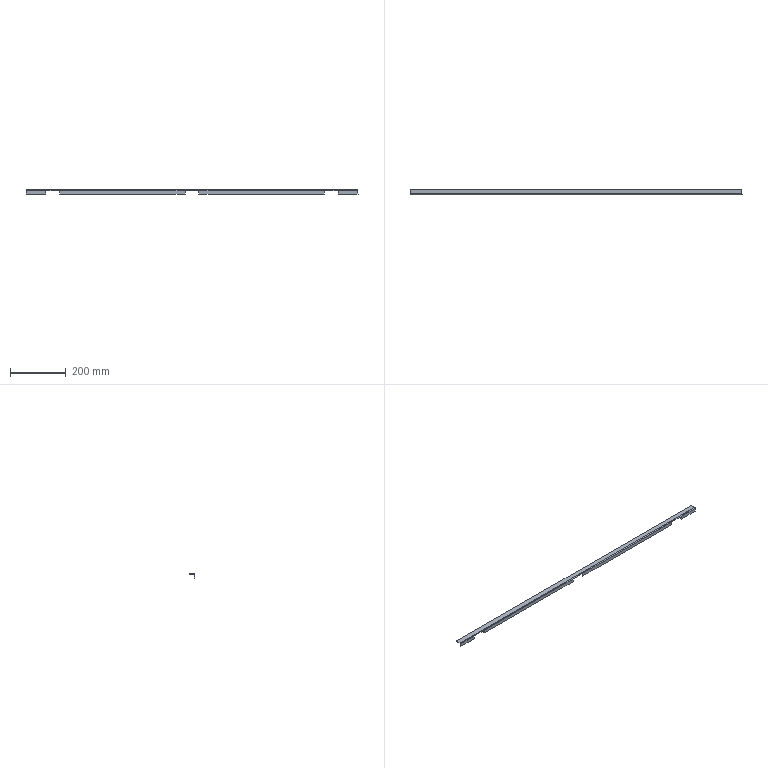Part | SolidWorks | features LPattern 2, Cut 1, EdgeFlange 1, FlatPattern 1, ICE 1, SMBaseFlange 1, SheetMetal 1 | 1 solid | 32 faces | box 1191 x 20 x 15 mm | volume 90032 mm3 | plane 30 | cylinder 2 | commonest cylinder face diameters 1 x1 6 x1
STEP:
#1=CARTESIAN_POINT('',(475.,-10.,-3.));
#2=VERTEX_POINT('',#1);
#3=CARTESIAN_POINT('',(25.,-10.,-3.));
#4=VERTEX_POINT('',#3);
#5=CARTESIAN_POINT('',(-595.5,-10.,-3.));
#6=DIRECTION('',(-1.,0.,0.));
#7=VECTOR('',#6,1000.);
#8=LINE('',#5,#7);
#9=EDGE_CURVE('',#2,#4,#8,.T.);
#10=ORIENTED_EDGE('',*,*,#9,.T.);
#11=CARTESIAN_POINT('',(25.,-10.,-15.));
#12=VERTEX_POINT('',#11);
#13=CARTESIAN_POINT('',(25.,-10.,-2.5));
#14=DIRECTION('',(0.,0.,-1.));
#15=VECTOR('',#14,1000.);
#16=LINE('',#13,#15);
#17=EDGE_CURVE('',#4,#12,#16,.T.);
#18=ORIENTED_EDGE('',*,*,#17,.T.);
#19=CARTESIAN_POINT('',(475.,-10.,-15.));
#20=VERTEX_POINT('',#19);
#21=CARTESIAN_POINT('',(-595.5,-10.,-15.));
#22=DIRECTION('',(-1.,0.,0.));
#23=VECTOR('',#22,1000.);
#24=LINE('',#21,#23);
#25=EDGE_CURVE('',#20,#12,#24,.T.);
#26=ORIENTED_EDGE('',*,*,#25,.F.);
#27=CARTESIAN_POINT('',(475.,-10.,-2.5));
#28=DIRECTION('',(0.,0.,1.));
#29=VECTOR('',#28,1000.);
#30=LINE('',#27,#29);
#31=EDGE_CURVE('',#20,#2,#30,.T.);
#32=ORIENTED_EDGE('',*,*,#31,.T.);
#33=EDGE_LOOP('',(#10,#18,#26,#32));
#34=FACE_OUTER_BOUND('',#33,.T.);
#35=CARTESIAN_POINT('',(-595.5,-10.,-2.5));
#36=DIRECTION('',(0.,-1.,0.));
#37=DIRECTION('',(0.,0.,-1.));
#38=AXIS2_PLACEMENT_3D('',#35,#36,#37);
#39=PLANE('',#38);
#40=ADVANCED_FACE('',(#34),#39,.T.);
#41=CARTESIAN_POINT('',(-25.,-10.,-15.));
#42=VERTEX_POINT('',#41);
#43=CARTESIAN_POINT('',(-475.,-10.,-15.));
#44=VERTEX_POINT('',#43);
#45=CARTESIAN_POINT('',(-595.5,-10.,-15.));
#46=DIRECTION('',(-1.,0.,0.));
#47=VECTOR('',#46,1000.);
#48=LINE('',#45,#47);
#49=EDGE_CURVE('',#42,#44,#48,.T.);
#50=ORIENTED_EDGE('',*,*,#49,.F.);
#51=CARTESIAN_POINT('',(-25.,-10.,-3.));
#52=VERTEX_POINT('',#51);
#53=CARTESIAN_POINT('',(-25.,-10.,-2.5));
#54=DIRECTION('',(0.,0.,1.));
#55=VECTOR('',#54,1000.);
#56=LINE('',#53,#55);
#57=EDGE_CURVE('',#42,#52,#56,.T.);
#58=ORIENTED_EDGE('',*,*,#57,.T.);
#59=CARTESIAN_POINT('',(-475.,-10.,-3.));
#60=VERTEX_POINT('',#59);
#61=CARTESIAN_POINT('',(-595.5,-10.,-3.));
#62=DIRECTION('',(-1.,0.,0.));
#63=VECTOR('',#62,1000.);
#64=LINE('',#61,#63);
#65=EDGE_CURVE('',#52,#60,#64,.T.);
#66=ORIENTED_EDGE('',*,*,#65,.T.);
#67=CARTESIAN_POINT('',(-475.,-10.,-2.5));
#68=DIRECTION('',(0.,0.,-1.));
#69=VECTOR('',#68,1000.);
#70=LINE('',#67,#69);
#71=EDGE_CURVE('',#60,#44,#70,.T.);
#72=ORIENTED_EDGE('',*,*,#71,.T.);
#73=EDGE_LOOP('',(#50,#58,#66,#72));
#74=FACE_OUTER_BOUND('',#73,.T.);
#75=CARTESIAN_POINT('',(-595.5,-10.,-2.5));
#76=DIRECTION('',(0.,-1.,0.));
#77=DIRECTION('',(0.,0.,-1.));
#78=AXIS2_PLACEMENT_3D('',#75,#76,#77);
#79=PLANE('',#78);
#80=ADVANCED_FACE('',(#74),#79,.T.);
#81=CARTESIAN_POINT('',(25.,-7.5,-3.));
#82=VERTEX_POINT('',#81);
#83=CARTESIAN_POINT('',(25.,-7.5,-15.));
#84=VERTEX_POINT('',#83);
#85=CARTESIAN_POINT('',(25.,-7.5,-3.));
#86=DIRECTION('',(0.,0.,-1.));
#87=VECTOR('',#86,1000.);
#88=LINE('',#85,#87);
#89=EDGE_CURVE('',#82,#84,#88,.T.);
#90=ORIENTED_EDGE('',*,*,#89,.F.);
#91=CARTESIAN_POINT('',(475.,-7.5,-3.));
#92=VERTEX_POINT('',#91);
#93=CARTESIAN_POINT('',(595.5,-7.5,-3.));
#94=DIRECTION('',(-1.,0.,0.));
#95=VECTOR('',#94,1000.);
#96=LINE('',#93,#95);
#97=EDGE_CURVE('',#92,#82,#96,.T.);
#98=ORIENTED_EDGE('',*,*,#97,.F.);
#99=CARTESIAN_POINT('',(475.,-7.5,-15.));
#100=VERTEX_POINT('',#99);
#101=CARTESIAN_POINT('',(475.,-7.5,-3.));
#102=DIRECTION('',(0.,0.,1.));
#103=VECTOR('',#102,1000.);
#104=LINE('',#101,#103);
#105=EDGE_CURVE('',#100,#92,#104,.T.);
#106=ORIENTED_EDGE('',*,*,#105,.F.);
#107=CARTESIAN_POINT('',(-595.5,-7.5,-15.));
#108=DIRECTION('',(-1.,0.,0.));
#109=VECTOR('',#108,1000.);
#110=LINE('',#107,#109);
#111=EDGE_CURVE('',#100,#84,#110,.T.);
#112=ORIENTED_EDGE('',*,*,#111,.T.);
#113=EDGE_LOOP('',(#90,#98,#106,#112));
#114=FACE_OUTER_BOUND('',#113,.T.);
#115=CARTESIAN_POINT('',(-595.5,-7.5,-2.5));
#116=DIRECTION('',(0.,-1.,0.));
#117=DIRECTION('',(0.,0.,-1.));
#118=AXIS2_PLACEMENT_3D('',#115,#116,#117);
#119=PLANE('',#118);
#120=ADVANCED_FACE('',(#114),#119,.F.);
#121=CARTESIAN_POINT('',(-25.,-7.5,-15.));
#122=VERTEX_POINT('',#121);
#123=CARTESIAN_POINT('',(-25.,-7.5,-3.));
#124=VERTEX_POINT('',#123);
#125=CARTESIAN_POINT('',(-25.,-7.5,-3.));
#126=DIRECTION('',(0.,0.,1.));
#127=VECTOR('',#126,1000.);
#128=LINE('',#125,#127);
#129=EDGE_CURVE('',#122,#124,#128,.T.);
#130=ORIENTED_EDGE('',*,*,#129,.F.);
#131=CARTESIAN_POINT('',(-475.,-7.5,-15.));
#132=VERTEX_POINT('',#131);
#133=CARTESIAN_POINT('',(-595.5,-7.5,-15.));
#134=DIRECTION('',(-1.,0.,0.));
#135=VECTOR('',#134,1000.);
#136=LINE('',#133,#135);
#137=EDGE_CURVE('',#122,#132,#136,.T.);
#138=ORIENTED_EDGE('',*,*,#137,.T.);
#139=CARTESIAN_POINT('',(-475.,-7.5,-3.));
#140=VERTEX_POINT('',#139);
#141=CARTESIAN_POINT('',(-475.,-7.5,-3.));
#142=DIRECTION('',(0.,0.,-1.));
#143=VECTOR('',#142,1000.);
#144=LINE('',#141,#143);
#145=EDGE_CURVE('',#140,#132,#144,.T.);
#146=ORIENTED_EDGE('',*,*,#145,.F.);
#147=CARTESIAN_POINT('',(595.5,-7.5,-3.));
#148=DIRECTION('',(-1.,0.,0.));
#149=VECTOR('',#148,1000.);
#150=LINE('',#147,#149);
#151=EDGE_CURVE('',#124,#140,#150,.T.);
#152=ORIENTED_EDGE('',*,*,#151,.F.);
#153=EDGE_LOOP('',(#130,#138,#146,#152));
#154=FACE_OUTER_BOUND('',#153,.T.);
#155=CARTESIAN_POINT('',(-595.5,-7.5,-2.5));
#156=DIRECTION('',(0.,-1.,0.));
#157=DIRECTION('',(0.,0.,-1.));
#158=AXIS2_PLACEMENT_3D('',#155,#156,#157);
#159=PLANE('',#158);
#160=ADVANCED_FACE('',(#154),#159,.F.);
#161=ORIENTED_EDGE('',*,*,#25,.T.);
#162=CARTESIAN_POINT('',(25.,-7.5,-15.));
#163=DIRECTION('',(0.,-1.,0.));
#164=VECTOR('',#163,1000.);
#165=LINE('',#162,#164);
#166=EDGE_CURVE('',#84,#12,#165,.T.);
#167=ORIENTED_EDGE('',*,*,#166,.F.);
#168=ORIENTED_EDGE('',*,*,#111,.F.);
#169=CARTESIAN_POINT('',(475.,-7.5,-15.));
#170=DIRECTION('',(0.,-1.,0.));
#171=VECTOR('',#170,1000.);
#172=LINE('',#169,#171);
#173=EDGE_CURVE('',#100,#20,#172,.T.);
#174=ORIENTED_EDGE('',*,*,#173,.T.);
#175=EDGE_LOOP('',(#161,#167,#168,#174));
#176=FACE_OUTER_BOUND('',#175,.T.);
#177=CARTESIAN_POINT('',(-595.5,-10.,-15.));
#178=DIRECTION('',(0.,0.,-1.));
#179=DIRECTION('',(0.,1.,0.));
#180=AXIS2_PLACEMENT_3D('',#177,#178,#179);
#181=PLANE('',#180);
#182=ADVANCED_FACE('',(#176),#181,.T.);
#183=ORIENTED_EDGE('',*,*,#137,.F.);
#184=CARTESIAN_POINT('',(-25.,-7.5,-15.));
#185=DIRECTION('',(0.,-1.,0.));
#186=VECTOR('',#185,1000.);
#187=LINE('',#184,#186);
#188=EDGE_CURVE('',#122,#42,#187,.T.);
#189=ORIENTED_EDGE('',*,*,#188,.T.);
#190=ORIENTED_EDGE('',*,*,#49,.T.);
#191=CARTESIAN_POINT('',(-475.,-7.5,-15.));
#192=DIRECTION('',(0.,-1.,0.));
#193=VECTOR('',#192,1000.);
#194=LINE('',#191,#193);
#195=EDGE_CURVE('',#132,#44,#194,.T.);
#196=ORIENTED_EDGE('',*,*,#195,.F.);
#197=EDGE_LOOP('',(#183,#189,#190,#196));
#198=FACE_OUTER_BOUND('',#197,.T.);
#199=CARTESIAN_POINT('',(-595.5,-10.,-15.));
#200=DIRECTION('',(0.,0.,-1.));
#201=DIRECTION('',(0.,1.,0.));
#202=AXIS2_PLACEMENT_3D('',#199,#200,#201);
#203=PLANE('',#202);
#204=ADVANCED_FACE('',(#198),#203,.T.);
#205=CARTESIAN_POINT('',(595.5,-10.,-3.));
#206=VERTEX_POINT('',#205);
#207=CARTESIAN_POINT('',(525.,-10.,-3.));
#208=VERTEX_POINT('',#207);
#209=CARTESIAN_POINT('',(-595.5,-10.,-3.));
#210=DIRECTION('',(-1.,0.,0.));
#211=VECTOR('',#210,1000.);
#212=LINE('',#209,#211);
#213=EDGE_CURVE('',#206,#208,#212,.T.);
#214=ORIENTED_EDGE('',*,*,#213,.T.);
#215=CARTESIAN_POINT('',(525.,-10.,-15.));
#216=VERTEX_POINT('',#215);
#217=CARTESIAN_POINT('',(525.,-10.,-2.5));
#218=DIRECTION('',(0.,0.,-1.));
#219=VECTOR('',#218,1000.);
#220=LINE('',#217,#219);
#221=EDGE_CURVE('',#208,#216,#220,.T.);
#222=ORIENTED_EDGE('',*,*,#221,.T.);
#223=CARTESIAN_POINT('',(595.5,-10.,-15.));
#224=VERTEX_POINT('',#223);
#225=CARTESIAN_POINT('',(-595.5,-10.,-15.));
#226=DIRECTION('',(-1.,0.,0.));
#227=VECTOR('',#226,1000.);
#228=LINE('',#225,#227);
#229=EDGE_CURVE('',#224,#216,#228,.T.);
#230=ORIENTED_EDGE('',*,*,#229,.F.);
#231=CARTESIAN_POINT('',(595.5,-10.,-15.));
#232=DIRECTION('',(0.,0.,-1.));
#233=VECTOR('',#232,1000.);
#234=LINE('',#231,#233);
#235=EDGE_CURVE('',#206,#224,#234,.T.);
#236=ORIENTED_EDGE('',*,*,#235,.F.);
#237=EDGE_LOOP('',(#214,#222,#230,#236));
#238=FACE_OUTER_BOUND('',#237,.T.);
#239=CARTESIAN_POINT('',(-595.5,-10.,-2.5));
#240=DIRECTION('',(0.,-1.,0.));
#241=DIRECTION('',(0.,0.,-1.));
#242=AXIS2_PLACEMENT_3D('',#239,#240,#241);
#243=PLANE('',#242);
#244=ADVANCED_FACE('',(#238),#243,.T.);
#245=CARTESIAN_POINT('',(525.,-7.5,-3.));
#246=VERTEX_POINT('',#245);
#247=CARTESIAN_POINT('',(525.,-7.5,-15.));
#248=VERTEX_POINT('',#247);
#249=CARTESIAN_POINT('',(525.,-7.5,-3.));
#250=DIRECTION('',(0.,0.,-1.));
#251=VECTOR('',#250,1000.);
#252=LINE('',#249,#251);
#253=EDGE_CURVE('',#246,#248,#252,.T.);
#254=ORIENTED_EDGE('',*,*,#253,.F.);
#255=CARTESIAN_POINT('',(595.5,-7.5,-3.));
#256=VERTEX_POINT('',#255);
#257=CARTESIAN_POINT('',(595.5,-7.5,-3.));
#258=DIRECTION('',(-1.,0.,0.));
#259=VECTOR('',#258,1000.);
#260=LINE('',#257,#259);
#261=EDGE_CURVE('',#256,#246,#260,.T.);
#262=ORIENTED_EDGE('',*,*,#261,.F.);
#263=CARTESIAN_POINT('',(595.5,-7.5,-15.));
#264=VERTEX_POINT('',#263);
#265=CARTESIAN_POINT('',(595.5,-7.5,-2.5));
#266=DIRECTION('',(0.,0.,-1.));
#267=VECTOR('',#266,1000.);
#268=LINE('',#265,#267);
#269=EDGE_CURVE('',#256,#264,#268,.T.);
#270=ORIENTED_EDGE('',*,*,#269,.T.);
#271=CARTESIAN_POINT('',(-595.5,-7.5,-15.));
#272=DIRECTION('',(-1.,0.,0.));
#273=VECTOR('',#272,1000.);
#274=LINE('',#271,#273);
#275=EDGE_CURVE('',#264,#248,#274,.T.);
#276=ORIENTED_EDGE('',*,*,#275,.T.);
#277=EDGE_LOOP('',(#254,#262,#270,#276));
#278=FACE_OUTER_BOUND('',#277,.T.);
#279=CARTESIAN_POINT('',(-595.5,-7.5,-2.5));
#280=DIRECTION('',(0.,-1.,0.));
#281=DIRECTION('',(0.,0.,-1.));
#282=AXIS2_PLACEMENT_3D('',#279,#280,#281);
#283=PLANE('',#282);
#284=ADVANCED_FACE('',(#278),#283,.F.);
#285=ORIENTED_EDGE('',*,*,#229,.T.);
#286=CARTESIAN_POINT('',(525.,-7.5,-15.));
#287=DIRECTION('',(0.,-1.,0.));
#288=VECTOR('',#287,1000.);
#289=LINE('',#286,#288);
#290=EDGE_CURVE('',#248,#216,#289,.T.);
#291=ORIENTED_EDGE('',*,*,#290,.F.);
#292=ORIENTED_EDGE('',*,*,#275,.F.);
#293=CARTESIAN_POINT('',(595.5,-10.,-15.));
#294=DIRECTION('',(0.,1.,0.));
#295=VECTOR('',#294,1000.);
#296=LINE('',#293,#295);
#297=EDGE_CURVE('',#224,#264,#296,.T.);
#298=ORIENTED_EDGE('',*,*,#297,.F.);
#299=EDGE_LOOP('',(#285,#291,#292,#298));
#300=FACE_OUTER_BOUND('',#299,.T.);
#301=CARTESIAN_POINT('',(-595.5,-10.,-15.));
#302=DIRECTION('',(0.,0.,-1.));
#303=DIRECTION('',(0.,1.,0.));
#304=AXIS2_PLACEMENT_3D('',#301,#302,#303);
#305=PLANE('',#304);
#306=ADVANCED_FACE('',(#300),#305,.T.);
#307=CARTESIAN_POINT('',(-525.,-10.,-15.));
#308=VERTEX_POINT('',#307);
#309=CARTESIAN_POINT('',(-595.5,-10.,-15.));
#310=VERTEX_POINT('',#309);
#311=CARTESIAN_POINT('',(-595.5,-10.,-15.));
#312=DIRECTION('',(-1.,0.,0.));
#313=VECTOR('',#312,1000.);
#314=LINE('',#311,#313);
#315=EDGE_CURVE('',#308,#310,#314,.T.);
#316=ORIENTED_EDGE('',*,*,#315,.F.);
#317=CARTESIAN_POINT('',(-525.,-10.,-3.));
#318=VERTEX_POINT('',#317);
#319=CARTESIAN_POINT('',(-525.,-10.,-2.5));
#320=DIRECTION('',(0.,0.,1.));
#321=VECTOR('',#320,1000.);
#322=LINE('',#319,#321);
#323=EDGE_CURVE('',#308,#318,#322,.T.);
#324=ORIENTED_EDGE('',*,*,#323,.T.);
#325=CARTESIAN_POINT('',(-595.5,-10.,-3.));
#326=VERTEX_POINT('',#325);
#327=CARTESIAN_POINT('',(-595.5,-10.,-3.));
#328=DIRECTION('',(-1.,0.,0.));
#329=VECTOR('',#328,1000.);
#330=LINE('',#327,#329);
#331=EDGE_CURVE('',#318,#326,#330,.T.);
#332=ORIENTED_EDGE('',*,*,#331,.T.);
#333=CARTESIAN_POINT('',(-595.5,-10.,-2.5));
#334=DIRECTION('',(0.,0.,1.));
#335=VECTOR('',#334,1000.);
#336=LINE('',#333,#335);
#337=EDGE_CURVE('',#310,#326,#336,.T.);
#338=ORIENTED_EDGE('',*,*,#337,.F.);
#339=EDGE_LOOP('',(#316,#324,#332,#338));
#340=FACE_OUTER_BOUND('',#339,.T.);
#341=CARTESIAN_POINT('',(-595.5,-10.,-2.5));
#342=DIRECTION('',(0.,-1.,0.));
#343=DIRECTION('',(0.,0.,-1.));
#344=AXIS2_PLACEMENT_3D('',#341,#342,#343);
#345=PLANE('',#344);
#346=ADVANCED_FACE('',(#340),#345,.T.);
#347=CARTESIAN_POINT('',(-525.,-7.5,-15.));
#348=VERTEX_POINT('',#347);
#349=CARTESIAN_POINT('',(-525.,-7.5,-3.));
#350=VERTEX_POINT('',#349);
#351=CARTESIAN_POINT('',(-525.,-7.5,-3.));
#352=DIRECTION('',(0.,0.,1.));
#353=VECTOR('',#352,1000.);
#354=LINE('',#351,#353);
#355=EDGE_CURVE('',#348,#350,#354,.T.);
#356=ORIENTED_EDGE('',*,*,#355,.F.);
#357=CARTESIAN_POINT('',(-595.5,-7.5,-15.));
#358=VERTEX_POINT('',#357);
#359=CARTESIAN_POINT('',(-595.5,-7.5,-15.));
#360=DIRECTION('',(-1.,0.,0.));
#361=VECTOR('',#360,1000.);
#362=LINE('',#359,#361);
#363=EDGE_CURVE('',#348,#358,#362,.T.);
#364=ORIENTED_EDGE('',*,*,#363,.T.);
#365=CARTESIAN_POINT('',(-595.5,-7.5,-3.));
#366=VERTEX_POINT('',#365);
#367=CARTESIAN_POINT('',(-595.5,-7.5,-2.5));
#368=DIRECTION('',(0.,0.,1.));
#369=VECTOR('',#368,1000.);
#370=LINE('',#367,#369);
#371=EDGE_CURVE('',#358,#366,#370,.T.);
#372=ORIENTED_EDGE('',*,*,#371,.T.);
#373=CARTESIAN_POINT('',(595.5,-7.5,-3.));
#374=DIRECTION('',(-1.,0.,0.));
#375=VECTOR('',#374,1000.);
#376=LINE('',#373,#375);
#377=EDGE_CURVE('',#350,#366,#376,.T.);
#378=ORIENTED_EDGE('',*,*,#377,.F.);
#379=EDGE_LOOP('',(#356,#364,#372,#378));
#380=FACE_OUTER_BOUND('',#379,.T.);
#381=CARTESIAN_POINT('',(-595.5,-7.5,-2.5));
#382=DIRECTION('',(0.,-1.,0.));
#383=DIRECTION('',(0.,0.,-1.));
#384=AXIS2_PLACEMENT_3D('',#381,#382,#383);
#385=PLANE('',#384);
#386=ADVANCED_FACE('',(#380),#385,.F.);
#387=ORIENTED_EDGE('',*,*,#363,.F.);
#388=CARTESIAN_POINT('',(-525.,-7.5,-15.));
#389=DIRECTION('',(0.,-1.,0.));
#390=VECTOR('',#389,1000.);
#391=LINE('',#388,#390);
#392=EDGE_CURVE('',#348,#308,#391,.T.);
#393=ORIENTED_EDGE('',*,*,#392,.T.);
#394=ORIENTED_EDGE('',*,*,#315,.T.);
#395=CARTESIAN_POINT('',(-595.5,-10.,-15.));
#396=DIRECTION('',(0.,1.,0.));
#397=VECTOR('',#396,1000.);
#398=LINE('',#395,#397);
#399=EDGE_CURVE('',#310,#358,#398,.T.);
#400=ORIENTED_EDGE('',*,*,#399,.T.);
#401=EDGE_LOOP('',(#387,#393,#394,#400));
#402=FACE_OUTER_BOUND('',#401,.T.);
#403=CARTESIAN_POINT('',(-595.5,-10.,-15.));
#404=DIRECTION('',(0.,0.,-1.));
#405=DIRECTION('',(0.,1.,0.));
#406=AXIS2_PLACEMENT_3D('',#403,#404,#405);
#407=PLANE('',#406);
#408=ADVANCED_FACE('',(#402),#407,.T.);
#409=CARTESIAN_POINT('',(-595.5,10.,-2.5));
#410=VERTEX_POINT('',#409);
#411=CARTESIAN_POINT('',(-595.5,-7.,-2.5));
#412=VERTEX_POINT('',#411);
#413=CARTESIAN_POINT('',(-595.5,-10.,-2.5));
#414=DIRECTION('',(0.,-1.,0.));
#415=VECTOR('',#414,1000.);
#416=LINE('',#413,#415);
#417=EDGE_CURVE('',#410,#412,#416,.T.);
#418=ORIENTED_EDGE('',*,*,#417,.T.);
#419=CARTESIAN_POINT('',(-595.5,-7.,0.));
#420=VERTEX_POINT('',#419);
#421=CARTESIAN_POINT('',(-595.5,-7.,-2.5));
#422=DIRECTION('',(0.,0.,1.));
#423=VECTOR('',#422,1000.);
#424=LINE('',#421,#423);
#425=EDGE_CURVE('',#412,#420,#424,.T.);
#426=ORIENTED_EDGE('',*,*,#425,.T.);
#427=CARTESIAN_POINT('',(-595.5,10.,0.));
#428=VERTEX_POINT('',#427);
#429=CARTESIAN_POINT('',(-595.5,-10.,0.));
#430=DIRECTION('',(0.,-1.,0.));
#431=VECTOR('',#430,1000.);
#432=LINE('',#429,#431);
#433=EDGE_CURVE('',#428,#420,#432,.T.);
#434=ORIENTED_EDGE('',*,*,#433,.F.);
#435=CARTESIAN_POINT('',(-595.5,10.,-2.5));
#436=DIRECTION('',(0.,0.,1.));
#437=VECTOR('',#436,1000.);
#438=LINE('',#435,#437);
#439=EDGE_CURVE('',#410,#428,#438,.T.);
#440=ORIENTED_EDGE('',*,*,#439,.F.);
#441=EDGE_LOOP('',(#418,#426,#434,#440));
#442=FACE_OUTER_BOUND('',#441,.T.);
#443=CARTESIAN_POINT('',(-595.5,-10.,-2.5));
#444=DIRECTION('',(-1.,0.,0.));
#445=DIRECTION('',(0.,0.,1.));
#446=AXIS2_PLACEMENT_3D('',#443,#444,#445);
#447=PLANE('',#446);
#448=ADVANCED_FACE('',(#442),#447,.T.);
#449=CARTESIAN_POINT('',(595.5,-7.,-2.5));
#450=VERTEX_POINT('',#449);
#451=CARTESIAN_POINT('',(595.5,10.,-2.5));
#452=VERTEX_POINT('',#451);
#453=CARTESIAN_POINT('',(595.5,-10.,-2.5));
#454=DIRECTION('',(0.,1.,0.));
#455=VECTOR('',#454,1000.);
#456=LINE('',#453,#455);
#457=EDGE_CURVE('',#450,#452,#456,.T.);
#458=ORIENTED_EDGE('',*,*,#457,.F.);
#459=CARTESIAN_POINT('',(-595.5,-7.,-2.5));
#460=DIRECTION('',(1.,0.,0.));
#461=VECTOR('',#460,1000.);
#462=LINE('',#459,#461);
#463=EDGE_CURVE('',#412,#450,#462,.T.);
#464=ORIENTED_EDGE('',*,*,#463,.F.);
#465=ORIENTED_EDGE('',*,*,#417,.F.);
#466=CARTESIAN_POINT('',(-595.5,10.,-2.5));
#467=DIRECTION('',(-1.,0.,0.));
#468=VECTOR('',#467,1000.);
#469=LINE('',#466,#468);
#470=EDGE_CURVE('',#452,#410,#469,.T.);
#471=ORIENTED_EDGE('',*,*,#470,.F.);
#472=EDGE_LOOP('',(#458,#464,#465,#471));
#473=FACE_OUTER_BOUND('',#472,.T.);
#474=CARTESIAN_POINT('',(595.5,10.,-2.5));
#475=DIRECTION('',(0.,0.,-1.));
#476=DIRECTION('',(-1.,0.,0.));
#477=AXIS2_PLACEMENT_3D('',#474,#475,#476);
#478=PLANE('',#477);
#479=ADVANCED_FACE('',(#473),#478,.T.);
#480=CARTESIAN_POINT('',(595.5,-7.,0.));
#481=VERTEX_POINT('',#480);
#482=CARTESIAN_POINT('',(-595.5,-7.,0.));
#483=DIRECTION('',(1.,0.,0.));
#484=VECTOR('',#483,1000.);
#485=LINE('',#482,#484);
#486=EDGE_CURVE('',#420,#481,#485,.T.);
#487=ORIENTED_EDGE('',*,*,#486,.T.);
#488=CARTESIAN_POINT('',(595.5,10.,0.));
#489=VERTEX_POINT('',#488);
#490=CARTESIAN_POINT('',(595.5,-10.,0.));
#491=DIRECTION('',(0.,1.,0.));
#492=VECTOR('',#491,1000.);
#493=LINE('',#490,#492);
#494=EDGE_CURVE('',#481,#489,#493,.T.);
#495=ORIENTED_EDGE('',*,*,#494,.T.);
#496=CARTESIAN_POINT('',(-595.5,10.,0.));
#497=DIRECTION('',(-1.,0.,0.));
#498=VECTOR('',#497,1000.);
#499=LINE('',#496,#498);
#500=EDGE_CURVE('',#489,#428,#499,.T.);
#501=ORIENTED_EDGE('',*,*,#500,.T.);
#502=ORIENTED_EDGE('',*,*,#433,.T.);
#503=EDGE_LOOP('',(#487,#495,#501,#502));
#504=FACE_OUTER_BOUND('',#503,.T.);
#505=CARTESIAN_POINT('',(595.5,10.,0.));
#506=DIRECTION('',(0.,0.,-1.));
#507=DIRECTION('',(-1.,0.,0.));
#508=AXIS2_PLACEMENT_3D('',#505,#506,#507);
#509=PLANE('',#508);
#510=ADVANCED_FACE('',(#504),#509,.F.);
#511=CARTESIAN_POINT('',(595.5,-7.,-2.5));
#512=DIRECTION('',(0.,0.,1.));
#513=VECTOR('',#512,1000.);
#514=LINE('',#511,#513);
#515=EDGE_CURVE('',#450,#481,#514,.T.);
#516=ORIENTED_EDGE('',*,*,#515,.F.);
#517=ORIENTED_EDGE('',*,*,#457,.T.);
#518=CARTESIAN_POINT('',(595.5,10.,-2.5));
#519=DIRECTION('',(0.,0.,1.));
#520=VECTOR('',#519,1000.);
#521=LINE('',#518,#520);
#522=EDGE_CURVE('',#452,#489,#521,.T.);
#523=ORIENTED_EDGE('',*,*,#522,.T.);
#524=ORIENTED_EDGE('',*,*,#494,.F.);
#525=EDGE_LOOP('',(#516,#517,#523,#524));
#526=FACE_OUTER_BOUND('',#525,.T.);
#527=CARTESIAN_POINT('',(595.5,-10.,-2.5));
#528=DIRECTION('',(1.,0.,0.));
#529=DIRECTION('',(0.,0.,-1.));
#530=AXIS2_PLACEMENT_3D('',#527,#528,#529);
#531=PLANE('',#530);
#532=ADVANCED_FACE('',(#526),#531,.T.);
#533=ORIENTED_EDGE('',*,*,#500,.F.);
#534=ORIENTED_EDGE('',*,*,#522,.F.);
#535=ORIENTED_EDGE('',*,*,#470,.T.);
#536=ORIENTED_EDGE('',*,*,#439,.T.);
#537=EDGE_LOOP('',(#533,#534,#535,#536));
#538=FACE_OUTER_BOUND('',#537,.T.);
#539=CARTESIAN_POINT('',(-595.5,10.,-2.5));
#540=DIRECTION('',(0.,1.,0.));
#541=DIRECTION('',(0.,0.,1.));
#542=AXIS2_PLACEMENT_3D('',#539,#540,#541);
#543=PLANE('',#542);
#544=ADVANCED_FACE('',(#538),#543,.T.);
#545=CARTESIAN_POINT('',(595.5,-10.,-3.));
#546=DIRECTION('',(0.,-1.,0.));
#547=VECTOR('',#546,1000.);
#548=LINE('',#545,#547);
#549=EDGE_CURVE('',#256,#206,#548,.T.);
#550=ORIENTED_EDGE('',*,*,#549,.F.);
#551=CARTESIAN_POINT('',(595.5,-7.,-3.));
#552=DIRECTION('',(1.,0.,0.));
#553=DIRECTION('',(0.,0.,1.));
#554=AXIS2_PLACEMENT_3D('',#551,#552,#553);
#555=CIRCLE('',#554,0.5);
#556=EDGE_CURVE('',#450,#256,#555,.T.);
#557=ORIENTED_EDGE('',*,*,#556,.F.);
#558=ORIENTED_EDGE('',*,*,#515,.T.);
#559=CARTESIAN_POINT('',(595.5,-7.,-3.));
#560=DIRECTION('',(1.,0.,0.));
#561=DIRECTION('',(0.,0.,1.));
#562=AXIS2_PLACEMENT_3D('',#559,#560,#561);
#563=CIRCLE('',#562,3.);
#564=EDGE_CURVE('',#481,#206,#563,.T.);
#565=ORIENTED_EDGE('',*,*,#564,.T.);
#566=EDGE_LOOP('',(#550,#557,#558,#565));
#567=FACE_OUTER_BOUND('',#566,.T.);
#568=CARTESIAN_POINT('',(595.5,-7.,-3.));
#569=DIRECTION('',(1.,0.,0.));
#570=DIRECTION('',(0.,0.,-1.));
#571=AXIS2_PLACEMENT_3D('',#568,#569,#570);
#572=PLANE('',#571);
#573=ADVANCED_FACE('',(#567),#572,.T.);
#574=ORIENTED_EDGE('',*,*,#486,.F.);
#575=CARTESIAN_POINT('',(-595.5,-7.,-3.));
#576=DIRECTION('',(-1.,0.,0.));
#577=DIRECTION('',(0.,0.,1.));
#578=AXIS2_PLACEMENT_3D('',#575,#576,#577);
#579=CIRCLE('',#578,3.);
#580=EDGE_CURVE('',#326,#420,#579,.T.);
#581=ORIENTED_EDGE('',*,*,#580,.F.);
#582=ORIENTED_EDGE('',*,*,#331,.F.);
#583=CARTESIAN_POINT('',(-595.5,-10.,-3.));
#584=DIRECTION('',(1.,0.,0.));
#585=VECTOR('',#584,1000.);
#586=LINE('',#583,#585);
#587=EDGE_CURVE('',#318,#60,#586,.T.);
#588=ORIENTED_EDGE('',*,*,#587,.T.);
#589=ORIENTED_EDGE('',*,*,#65,.F.);
#590=CARTESIAN_POINT('',(-595.5,-10.,-3.));
#591=DIRECTION('',(1.,0.,0.));
#592=VECTOR('',#591,1000.);
#593=LINE('',#590,#592);
#594=EDGE_CURVE('',#52,#4,#593,.T.);
#595=ORIENTED_EDGE('',*,*,#594,.T.);
#596=ORIENTED_EDGE('',*,*,#9,.F.);
#597=CARTESIAN_POINT('',(-595.5,-10.,-3.));
#598=DIRECTION('',(1.,0.,0.));
#599=VECTOR('',#598,1000.);
#600=LINE('',#597,#599);
#601=EDGE_CURVE('',#2,#208,#600,.T.);
#602=ORIENTED_EDGE('',*,*,#601,.T.);
#603=ORIENTED_EDGE('',*,*,#213,.F.);
#604=ORIENTED_EDGE('',*,*,#564,.F.);
#605=EDGE_LOOP('',(#574,#581,#582,#588,#589,#595,#596,#602,#603,#604));
#606=FACE_OUTER_BOUND('',#605,.T.);
#607=CARTESIAN_POINT('',(-595.5,-7.,-3.));
#608=DIRECTION('',(-1.,0.,0.));
#609=DIRECTION('',(0.,-1.,0.));
#610=AXIS2_PLACEMENT_3D('',#607,#608,#609);
#611=CYLINDRICAL_SURFACE('',#610,3.);
#612=ADVANCED_FACE('',(#606),#611,.T.);
#613=CARTESIAN_POINT('',(-595.5,-7.,-3.));
#614=DIRECTION('',(-1.,0.,0.));
#615=DIRECTION('',(0.,0.,1.));
#616=AXIS2_PLACEMENT_3D('',#613,#614,#615);
#617=CIRCLE('',#616,0.5);
#618=EDGE_CURVE('',#366,#412,#617,.T.);
#619=ORIENTED_EDGE('',*,*,#618,.F.);
#620=CARTESIAN_POINT('',(-595.5,-7.5,-3.));
#621=DIRECTION('',(0.,-1.,0.));
#622=VECTOR('',#621,1000.);
#623=LINE('',#620,#622);
#624=EDGE_CURVE('',#366,#326,#623,.T.);
#625=ORIENTED_EDGE('',*,*,#624,.T.);
#626=ORIENTED_EDGE('',*,*,#580,.T.);
#627=ORIENTED_EDGE('',*,*,#425,.F.);
#628=EDGE_LOOP('',(#619,#625,#626,#627));
#629=FACE_OUTER_BOUND('',#628,.T.);
#630=CARTESIAN_POINT('',(-595.5,-7.,-3.));
#631=DIRECTION('',(1.,0.,0.));
#632=DIRECTION('',(0.,0.,-1.));
#633=AXIS2_PLACEMENT_3D('',#630,#631,#632);
#634=PLANE('',#633);
#635=ADVANCED_FACE('',(#629),#634,.F.);
#636=ORIENTED_EDGE('',*,*,#463,.T.);
#637=ORIENTED_EDGE('',*,*,#556,.T.);
#638=ORIENTED_EDGE('',*,*,#261,.T.);
#639=CARTESIAN_POINT('',(475.,-7.5,-3.));
#640=DIRECTION('',(1.,0.,0.));
#641=VECTOR('',#640,1000.);
#642=LINE('',#639,#641);
#643=EDGE_CURVE('',#92,#246,#642,.T.);
#644=ORIENTED_EDGE('',*,*,#643,.F.);
#645=ORIENTED_EDGE('',*,*,#97,.T.);
#646=CARTESIAN_POINT('',(-25.,-7.5,-3.));
#647=DIRECTION('',(1.,0.,0.));
#648=VECTOR('',#647,1000.);
#649=LINE('',#646,#648);
#650=EDGE_CURVE('',#124,#82,#649,.T.);
#651=ORIENTED_EDGE('',*,*,#650,.F.);
#652=ORIENTED_EDGE('',*,*,#151,.T.);
#653=CARTESIAN_POINT('',(-525.,-7.5,-3.));
#654=DIRECTION('',(1.,0.,0.));
#655=VECTOR('',#654,1000.);
#656=LINE('',#653,#655);
#657=EDGE_CURVE('',#350,#140,#656,.T.);
#658=ORIENTED_EDGE('',*,*,#657,.F.);
#659=ORIENTED_EDGE('',*,*,#377,.T.);
#660=ORIENTED_EDGE('',*,*,#618,.T.);
#661=EDGE_LOOP('',(#636,#637,#638,#644,#645,#651,#652,#658,#659,#660));
#662=FACE_OUTER_BOUND('',#661,.T.);
#663=CARTESIAN_POINT('',(-595.5,-7.,-3.));
#664=DIRECTION('',(-1.,0.,0.));
#665=DIRECTION('',(0.,-1.,0.));
#666=AXIS2_PLACEMENT_3D('',#663,#664,#665);
#667=CYLINDRICAL_SURFACE('',#666,0.5);
#668=ADVANCED_FACE('',(#662),#667,.F.);
#669=ORIENTED_EDGE('',*,*,#337,.T.);
#670=ORIENTED_EDGE('',*,*,#624,.F.);
#671=ORIENTED_EDGE('',*,*,#371,.F.);
#672=ORIENTED_EDGE('',*,*,#399,.F.);
#673=EDGE_LOOP('',(#669,#670,#671,#672));
#674=FACE_OUTER_BOUND('',#673,.T.);
#675=CARTESIAN_POINT('',(-595.5,-10.,-2.5));
#676=DIRECTION('',(-1.,0.,0.));
#677=DIRECTION('',(0.,0.,1.));
#678=AXIS2_PLACEMENT_3D('',#675,#676,#677);
#679=PLANE('',#678);
#680=ADVANCED_FACE('',(#674),#679,.T.);
#681=ORIENTED_EDGE('',*,*,#269,.F.);
#682=ORIENTED_EDGE('',*,*,#549,.T.);
#683=ORIENTED_EDGE('',*,*,#235,.T.);
#684=ORIENTED_EDGE('',*,*,#297,.T.);
#685=EDGE_LOOP('',(#681,#682,#683,#684));
#686=FACE_OUTER_BOUND('',#685,.T.);
#687=CARTESIAN_POINT('',(595.5,-10.,-15.));
#688=DIRECTION('',(1.,0.,0.));
#689=DIRECTION('',(0.,0.,-1.));
#690=AXIS2_PLACEMENT_3D('',#687,#688,#689);
#691=PLANE('',#690);
#692=ADVANCED_FACE('',(#686),#691,.T.);
#693=CARTESIAN_POINT('',(-475.,-7.5,-3.));
#694=DIRECTION('',(0.,-1.,0.));
#695=VECTOR('',#694,1000.);
#696=LINE('',#693,#695);
#697=EDGE_CURVE('',#140,#60,#696,.T.);
#698=ORIENTED_EDGE('',*,*,#697,.F.);
#699=ORIENTED_EDGE('',*,*,#145,.T.);
#700=ORIENTED_EDGE('',*,*,#195,.T.);
#701=ORIENTED_EDGE('',*,*,#71,.F.);
#702=EDGE_LOOP('',(#698,#699,#700,#701));
#703=FACE_OUTER_BOUND('',#702,.T.);
#704=CARTESIAN_POINT('',(-475.,-7.5,-3.));
#705=DIRECTION('',(-1.,0.,0.));
#706=DIRECTION('',(0.,0.,-1.));
#707=AXIS2_PLACEMENT_3D('',#704,#705,#706);
#708=PLANE('',#707);
#709=ADVANCED_FACE('',(#703),#708,.T.);
#710=ORIENTED_EDGE('',*,*,#392,.F.);
#711=ORIENTED_EDGE('',*,*,#355,.T.);
#712=CARTESIAN_POINT('',(-525.,-7.5,-3.));
#713=DIRECTION('',(0.,-1.,0.));
#714=VECTOR('',#713,1000.);
#715=LINE('',#712,#714);
#716=EDGE_CURVE('',#350,#318,#715,.T.);
#717=ORIENTED_EDGE('',*,*,#716,.T.);
#718=ORIENTED_EDGE('',*,*,#323,.F.);
#719=EDGE_LOOP('',(#710,#711,#717,#718));
#720=FACE_OUTER_BOUND('',#719,.T.);
#721=CARTESIAN_POINT('',(-525.,-7.5,-3.));
#722=DIRECTION('',(1.,0.,0.));
#723=DIRECTION('',(0.,0.,1.));
#724=AXIS2_PLACEMENT_3D('',#721,#722,#723);
#725=PLANE('',#724);
#726=ADVANCED_FACE('',(#720),#725,.T.);
#727=ORIENTED_EDGE('',*,*,#657,.T.);
#728=ORIENTED_EDGE('',*,*,#697,.T.);
#729=ORIENTED_EDGE('',*,*,#587,.F.);
#730=ORIENTED_EDGE('',*,*,#716,.F.);
#731=EDGE_LOOP('',(#727,#728,#729,#730));
#732=FACE_OUTER_BOUND('',#731,.T.);
#733=CARTESIAN_POINT('',(-525.,-7.5,-3.));
#734=DIRECTION('',(0.,0.,-1.));
#735=DIRECTION('',(1.,0.,0.));
#736=AXIS2_PLACEMENT_3D('',#733,#734,#735);
#737=PLANE('',#736);
#738=ADVANCED_FACE('',(#732),#737,.T.);
#739=CARTESIAN_POINT('',(525.,-7.5,-3.));
#740=DIRECTION('',(0.,-1.,0.));
#741=VECTOR('',#740,1000.);
#742=LINE('',#739,#741);
#743=EDGE_CURVE('',#246,#208,#742,.T.);
#744=ORIENTED_EDGE('',*,*,#743,.F.);
#745=ORIENTED_EDGE('',*,*,#253,.T.);
#746=ORIENTED_EDGE('',*,*,#290,.T.);
#747=ORIENTED_EDGE('',*,*,#221,.F.);
#748=EDGE_LOOP('',(#744,#745,#746,#747));
#749=FACE_OUTER_BOUND('',#748,.T.);
#750=CARTESIAN_POINT('',(525.,-7.5,-3.));
#751=DIRECTION('',(-1.,0.,0.));
#752=DIRECTION('',(0.,0.,-1.));
#753=AXIS2_PLACEMENT_3D('',#750,#751,#752);
#754=PLANE('',#753);
#755=ADVANCED_FACE('',(#749),#754,.T.);
#756=ORIENTED_EDGE('',*,*,#173,.F.);
#757=ORIENTED_EDGE('',*,*,#105,.T.);
#758=CARTESIAN_POINT('',(475.,-7.5,-3.));
#759=DIRECTION('',(0.,-1.,0.));
#760=VECTOR('',#759,1000.);
#761=LINE('',#758,#760);
#762=EDGE_CURVE('',#92,#2,#761,.T.);
#763=ORIENTED_EDGE('',*,*,#762,.T.);
#764=ORIENTED_EDGE('',*,*,#31,.F.);
#765=EDGE_LOOP('',(#756,#757,#763,#764));
#766=FACE_OUTER_BOUND('',#765,.T.);
#767=CARTESIAN_POINT('',(475.,-7.5,-3.));
#768=DIRECTION('',(1.,0.,0.));
#769=DIRECTION('',(0.,0.,1.));
#770=AXIS2_PLACEMENT_3D('',#767,#768,#769);
#771=PLANE('',#770);
#772=ADVANCED_FACE('',(#766),#771,.T.);
#773=ORIENTED_EDGE('',*,*,#643,.T.);
#774=ORIENTED_EDGE('',*,*,#743,.T.);
#775=ORIENTED_EDGE('',*,*,#601,.F.);
#776=ORIENTED_EDGE('',*,*,#762,.F.);
#777=EDGE_LOOP('',(#773,#774,#775,#776));
#778=FACE_OUTER_BOUND('',#777,.T.);
#779=CARTESIAN_POINT('',(475.,-7.5,-3.));
#780=DIRECTION('',(0.,0.,-1.));
#781=DIRECTION('',(1.,0.,0.));
#782=AXIS2_PLACEMENT_3D('',#779,#780,#781);
#783=PLANE('',#782);
#784=ADVANCED_FACE('',(#778),#783,.T.);
#785=CARTESIAN_POINT('',(25.,-7.5,-3.));
#786=DIRECTION('',(0.,-1.,0.));
#787=VECTOR('',#786,1000.);
#788=LINE('',#785,#787);
#789=EDGE_CURVE('',#82,#4,#788,.T.);
#790=ORIENTED_EDGE('',*,*,#789,.F.);
#791=ORIENTED_EDGE('',*,*,#89,.T.);
#792=ORIENTED_EDGE('',*,*,#166,.T.);
#793=ORIENTED_EDGE('',*,*,#17,.F.);
#794=EDGE_LOOP('',(#790,#791,#792,#793));
#795=FACE_OUTER_BOUND('',#794,.T.);
#796=CARTESIAN_POINT('',(25.,-7.5,-3.));
#797=DIRECTION('',(-1.,0.,0.));
#798=DIRECTION('',(0.,0.,-1.));
#799=AXIS2_PLACEMENT_3D('',#796,#797,#798);
#800=PLANE('',#799);
#801=ADVANCED_FACE('',(#795),#800,.T.);
#802=ORIENTED_EDGE('',*,*,#188,.F.);
#803=ORIENTED_EDGE('',*,*,#129,.T.);
#804=CARTESIAN_POINT('',(-25.,-7.5,-3.));
#805=DIRECTION('',(0.,-1.,0.));
#806=VECTOR('',#805,1000.);
#807=LINE('',#804,#806);
#808=EDGE_CURVE('',#124,#52,#807,.T.);
#809=ORIENTED_EDGE('',*,*,#808,.T.);
#810=ORIENTED_EDGE('',*,*,#57,.F.);
#811=EDGE_LOOP('',(#802,#803,#809,#810));
#812=FACE_OUTER_BOUND('',#811,.T.);
#813=CARTESIAN_POINT('',(-25.,-7.5,-3.));
#814=DIRECTION('',(1.,0.,0.));
#815=DIRECTION('',(0.,0.,1.));
#816=AXIS2_PLACEMENT_3D('',#813,#814,#815);
#817=PLANE('',#816);
#818=ADVANCED_FACE('',(#812),#817,.T.);
#819=ORIENTED_EDGE('',*,*,#650,.T.);
#820=ORIENTED_EDGE('',*,*,#789,.T.);
#821=ORIENTED_EDGE('',*,*,#594,.F.);
#822=ORIENTED_EDGE('',*,*,#808,.F.);
#823=EDGE_LOOP('',(#819,#820,#821,#822));
#824=FACE_OUTER_BOUND('',#823,.T.);
#825=CARTESIAN_POINT('',(-25.,-7.5,-3.));
#826=DIRECTION('',(0.,0.,-1.));
#827=DIRECTION('',(1.,0.,0.));
#828=AXIS2_PLACEMENT_3D('',#825,#826,#827);
#829=PLANE('',#828);
#830=ADVANCED_FACE('',(#824),#829,.T.);
#831=CLOSED_SHELL('',(#40,#80,#120,#160,#182,#204,#244,#284,#306,#346,#386,#408,#448,#479,#510,#532,#544,#573,#612,#635,#668,#680,#692,#709,#726,#738,#755,#772,#784,#801,#818,#830));
#832=MANIFOLD_SOLID_BREP('',#831);
#833=CARTESIAN_POINT('',(0.,0.,0.));
#834=DIRECTION('',(0.,0.,1.));
#835=DIRECTION('',(1.,0.,0.));
#836=AXIS2_PLACEMENT_3D('',#833,#834,#835);
#837=(LENGTH_UNIT()NAMED_UNIT(*)SI_UNIT(.MILLI.,.METRE.));
#838=UNCERTAINTY_MEASURE_WITH_UNIT(LENGTH_MEASURE(0.00001),#837,'','');
#839=(NAMED_UNIT(*)PLANE_ANGLE_UNIT()SI_UNIT($,.RADIAN.));
#840=(NAMED_UNIT(*)SI_UNIT($,.STERADIAN.)SOLID_ANGLE_UNIT());
#841=(GEOMETRIC_REPRESENTATION_CONTEXT(3)GLOBAL_UNCERTAINTY_ASSIGNED_CONTEXT((#838))GLOBAL_UNIT_ASSIGNED_CONTEXT((#837,#839,#840))REPRESENTATION_CONTEXT('',''));
#842=ADVANCED_BREP_SHAPE_REPRESENTATION('',(#832,#836),#841);